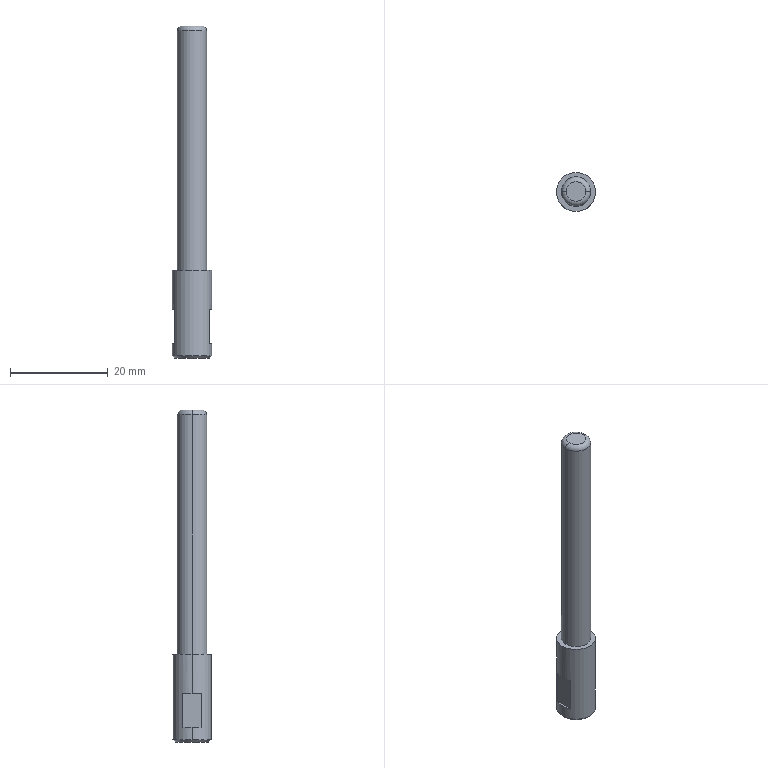Part | SolidWorks | features ICE 2, Chamfer 1, Extrusion 1, Fillet 1, HoleWzd 1 | 1 solid | 21 faces | box 8 x 8 x 68 mm | volume 2175 mm3 | plane 9 | cylinder 6 | cone 4 | torus 2 | commonest cylinder face diameters 3.3 x2 6 x2 8 x2
STEP:
#1=CARTESIAN_POINT('',(1.65,0.,13.5));
#2=VERTEX_POINT('',#1);
#3=CARTESIAN_POINT('',(-1.65,0.,13.5));
#4=VERTEX_POINT('',#3);
#5=CARTESIAN_POINT('',(0.,0.,13.5));
#6=DIRECTION('',(0.,0.,-1.));
#7=DIRECTION('',(-1.,0.,0.));
#8=AXIS2_PLACEMENT_3D('',#5,#6,#7);
#9=CIRCLE('',#8,1.65);
#10=EDGE_CURVE('',#2,#4,#9,.T.);
#11=ORIENTED_EDGE('',*,*,#10,.F.);
#12=CARTESIAN_POINT('',(1.65,0.,0.));
#13=VERTEX_POINT('',#12);
#14=CARTESIAN_POINT('',(1.65,0.,0.));
#15=DIRECTION('',(0.,0.,-1.));
#16=VECTOR('',#15,1000.);
#17=LINE('',#14,#16);
#18=EDGE_CURVE('',#2,#13,#17,.T.);
#19=ORIENTED_EDGE('',*,*,#18,.T.);
#20=CARTESIAN_POINT('',(-1.65,0.,0.));
#21=VERTEX_POINT('',#20);
#22=CARTESIAN_POINT('',(0.,0.,0.));
#23=DIRECTION('',(0.,0.,-1.));
#24=DIRECTION('',(-1.,0.,0.));
#25=AXIS2_PLACEMENT_3D('',#22,#23,#24);
#26=CIRCLE('',#25,1.65);
#27=EDGE_CURVE('',#13,#21,#26,.T.);
#28=ORIENTED_EDGE('',*,*,#27,.T.);
#29=CARTESIAN_POINT('',(-1.65,0.,0.));
#30=DIRECTION('',(0.,0.,-1.));
#31=VECTOR('',#30,1000.);
#32=LINE('',#29,#31);
#33=EDGE_CURVE('',#4,#21,#32,.T.);
#34=ORIENTED_EDGE('',*,*,#33,.F.);
#35=EDGE_LOOP('',(#11,#19,#28,#34));
#36=FACE_OUTER_BOUND('',#35,.T.);
#37=CARTESIAN_POINT('',(0.,0.,0.));
#38=DIRECTION('',(0.,0.,-1.));
#39=DIRECTION('',(-1.,0.,0.));
#40=AXIS2_PLACEMENT_3D('',#37,#38,#39);
#41=CYLINDRICAL_SURFACE('',#40,1.65);
#42=ADVANCED_FACE('',(#36),#41,.F.);
#43=CARTESIAN_POINT('',(0.,0.,14.491));
#44=VERTEX_POINT('',#43);
#45=CARTESIAN_POINT('',(-1.65,0.,13.5));
#46=DIRECTION('',(-0.8572,0.,-0.515));
#47=VECTOR('',#46,1000.);
#48=LINE('',#45,#47);
#49=EDGE_CURVE('',#44,#4,#48,.T.);
#50=ORIENTED_EDGE('',*,*,#49,.F.);
#51=CARTESIAN_POINT('',(1.65,0.,13.5));
#52=DIRECTION('',(0.8572,0.,-0.515));
#53=VECTOR('',#52,1000.);
#54=LINE('',#51,#53);
#55=EDGE_CURVE('',#44,#2,#54,.T.);
#56=ORIENTED_EDGE('',*,*,#55,.T.);
#57=ORIENTED_EDGE('',*,*,#10,.T.);
#58=EDGE_LOOP('',(#50,#56,#57));
#59=FACE_OUTER_BOUND('',#58,.T.);
#60=CARTESIAN_POINT('',(0.,0.,13.5));
#61=DIRECTION('',(0.,0.,-1.));
#62=DIRECTION('',(-1.,0.,0.));
#63=AXIS2_PLACEMENT_3D('',#60,#61,#62);
#64=CONICAL_SURFACE('',#63,1.65,1.03);
#65=ADVANCED_FACE('',(#59),#64,.F.);
#66=CARTESIAN_POINT('',(-3.5,0.,0.));
#67=VERTEX_POINT('',#66);
#68=CARTESIAN_POINT('',(3.5,0.,0.));
#69=VERTEX_POINT('',#68);
#70=CARTESIAN_POINT('',(0.,0.,0.));
#71=DIRECTION('',(0.,0.,-1.));
#72=DIRECTION('',(1.,0.,0.));
#73=AXIS2_PLACEMENT_3D('',#70,#71,#72);
#74=CIRCLE('',#73,3.5);
#75=EDGE_CURVE('',#67,#69,#74,.T.);
#76=ORIENTED_EDGE('',*,*,#75,.F.);
#77=CARTESIAN_POINT('',(-4.,0.,0.5));
#78=VERTEX_POINT('',#77);
#79=CARTESIAN_POINT('',(-4.,0.,0.5));
#80=DIRECTION('',(-0.7071,0.,0.7071));
#81=VECTOR('',#80,1000.);
#82=LINE('',#79,#81);
#83=EDGE_CURVE('',#67,#78,#82,.T.);
#84=ORIENTED_EDGE('',*,*,#83,.T.);
#85=CARTESIAN_POINT('',(4.,0.,0.5));
#86=VERTEX_POINT('',#85);
#87=CARTESIAN_POINT('',(0.,0.,0.5));
#88=DIRECTION('',(0.,0.,1.));
#89=DIRECTION('',(1.,0.,0.));
#90=AXIS2_PLACEMENT_3D('',#87,#88,#89);
#91=CIRCLE('',#90,4.);
#92=EDGE_CURVE('',#86,#78,#91,.T.);
#93=ORIENTED_EDGE('',*,*,#92,.F.);
#94=CARTESIAN_POINT('',(4.,0.,0.5));
#95=DIRECTION('',(0.7071,0.,0.7071));
#96=VECTOR('',#95,1000.);
#97=LINE('',#94,#96);
#98=EDGE_CURVE('',#69,#86,#97,.T.);
#99=ORIENTED_EDGE('',*,*,#98,.F.);
#100=EDGE_LOOP('',(#76,#84,#93,#99));
#101=FACE_OUTER_BOUND('',#100,.T.);
#102=CARTESIAN_POINT('',(0.,0.,0.5));
#103=DIRECTION('',(0.,0.,1.));
#104=DIRECTION('',(1.,0.,0.));
#105=AXIS2_PLACEMENT_3D('',#102,#103,#104);
#106=CONICAL_SURFACE('',#105,4.,0.7854);
#107=ADVANCED_FACE('',(#101),#106,.T.);
#108=CARTESIAN_POINT('',(-3.,0.,67.));
#109=VERTEX_POINT('',#108);
#110=CARTESIAN_POINT('',(3.,0.,67.));
#111=VERTEX_POINT('',#110);
#112=CARTESIAN_POINT('',(0.,0.,67.));
#113=DIRECTION('',(0.,0.,-1.));
#114=DIRECTION('',(1.,0.,0.));
#115=AXIS2_PLACEMENT_3D('',#112,#113,#114);
#116=CIRCLE('',#115,3.);
#117=EDGE_CURVE('',#109,#111,#116,.T.);
#118=ORIENTED_EDGE('',*,*,#117,.F.);
#119=CARTESIAN_POINT('',(-2.,0.,68.));
#120=VERTEX_POINT('',#119);
#121=CARTESIAN_POINT('',(-2.,0.,67.));
#122=DIRECTION('',(0.,1.,0.));
#123=DIRECTION('',(-1.,0.,0.));
#124=AXIS2_PLACEMENT_3D('',#121,#122,#123);
#125=CIRCLE('',#124,1.);
#126=EDGE_CURVE('',#109,#120,#125,.T.);
#127=ORIENTED_EDGE('',*,*,#126,.T.);
#128=CARTESIAN_POINT('',(2.,0.,68.));
#129=VERTEX_POINT('',#128);
#130=CARTESIAN_POINT('',(0.,0.,68.));
#131=DIRECTION('',(0.,0.,1.));
#132=DIRECTION('',(1.,0.,0.));
#133=AXIS2_PLACEMENT_3D('',#130,#131,#132);
#134=CIRCLE('',#133,2.);
#135=EDGE_CURVE('',#129,#120,#134,.T.);
#136=ORIENTED_EDGE('',*,*,#135,.F.);
#137=CARTESIAN_POINT('',(2.,0.,67.));
#138=DIRECTION('',(0.,-1.,0.));
#139=DIRECTION('',(0.,0.,-1.));
#140=AXIS2_PLACEMENT_3D('',#137,#138,#139);
#141=CIRCLE('',#140,1.);
#142=EDGE_CURVE('',#111,#129,#141,.T.);
#143=ORIENTED_EDGE('',*,*,#142,.F.);
#144=EDGE_LOOP('',(#118,#127,#136,#143));
#145=FACE_OUTER_BOUND('',#144,.T.);
#146=CARTESIAN_POINT('',(0.,0.,67.));
#147=DIRECTION('',(0.,0.,1.));
#148=DIRECTION('',(1.,0.,0.));
#149=AXIS2_PLACEMENT_3D('',#146,#147,#148);
#150=TOROIDAL_SURFACE('',#149,2.,1.);
#151=ADVANCED_FACE('',(#145),#150,.T.);
#152=ORIENTED_EDGE('',*,*,#117,.T.);
#153=CARTESIAN_POINT('',(3.,0.,18.));
#154=VERTEX_POINT('',#153);
#155=CARTESIAN_POINT('',(3.,0.,68.));
#156=DIRECTION('',(0.,0.,-1.));
#157=VECTOR('',#156,1000.);
#158=LINE('',#155,#157);
#159=EDGE_CURVE('',#111,#154,#158,.T.);
#160=ORIENTED_EDGE('',*,*,#159,.T.);
#161=CARTESIAN_POINT('',(-3.,0.,18.));
#162=VERTEX_POINT('',#161);
#163=CARTESIAN_POINT('',(0.,0.,18.));
#164=DIRECTION('',(0.,0.,1.));
#165=DIRECTION('',(1.,0.,0.));
#166=AXIS2_PLACEMENT_3D('',#163,#164,#165);
#167=CIRCLE('',#166,3.);
#168=EDGE_CURVE('',#154,#162,#167,.T.);
#169=ORIENTED_EDGE('',*,*,#168,.T.);
#170=CARTESIAN_POINT('',(-3.,0.,68.));
#171=DIRECTION('',(0.,0.,-1.));
#172=VECTOR('',#171,1000.);
#173=LINE('',#170,#172);
#174=EDGE_CURVE('',#109,#162,#173,.T.);
#175=ORIENTED_EDGE('',*,*,#174,.F.);
#176=EDGE_LOOP('',(#152,#160,#169,#175));
#177=FACE_OUTER_BOUND('',#176,.T.);
#178=CARTESIAN_POINT('',(0.,0.,68.));
#179=DIRECTION('',(0.,0.,-1.));
#180=DIRECTION('',(-1.,0.,0.));
#181=AXIS2_PLACEMENT_3D('',#178,#179,#180);
#182=CYLINDRICAL_SURFACE('',#181,3.);
#183=ADVANCED_FACE('',(#177),#182,.T.);
#184=CARTESIAN_POINT('',(4.,0.,18.));
#185=VERTEX_POINT('',#184);
#186=CARTESIAN_POINT('',(-4.,0.,18.));
#187=VERTEX_POINT('',#186);
#188=CARTESIAN_POINT('',(0.,0.,18.));
#189=DIRECTION('',(0.,0.,1.));
#190=DIRECTION('',(1.,0.,0.));
#191=AXIS2_PLACEMENT_3D('',#188,#189,#190);
#192=CIRCLE('',#191,4.);
#193=EDGE_CURVE('',#185,#187,#192,.T.);
#194=ORIENTED_EDGE('',*,*,#193,.F.);
#195=CARTESIAN_POINT('',(4.,0.,10.));
#196=VERTEX_POINT('',#195);
#197=CARTESIAN_POINT('',(4.,0.,18.));
#198=DIRECTION('',(0.,0.,-1.));
#199=VECTOR('',#198,1000.);
#200=LINE('',#197,#199);
#201=EDGE_CURVE('',#185,#196,#200,.T.);
#202=ORIENTED_EDGE('',*,*,#201,.T.);
#203=CARTESIAN_POINT('',(3.5,1.936,10.));
#204=VERTEX_POINT('',#203);
#205=CARTESIAN_POINT('',(0.,0.,10.));
#206=DIRECTION('',(0.,0.,-1.));
#207=DIRECTION('',(-1.,0.,0.));
#208=AXIS2_PLACEMENT_3D('',#205,#206,#207);
#209=CIRCLE('',#208,4.);
#210=EDGE_CURVE('',#204,#196,#209,.T.);
#211=ORIENTED_EDGE('',*,*,#210,.F.);
#212=CARTESIAN_POINT('',(3.5,1.936,3.));
#213=VERTEX_POINT('',#212);
#214=CARTESIAN_POINT('',(3.5,1.936,18.));
#215=DIRECTION('',(0.,0.,-1.));
#216=VECTOR('',#215,1000.);
#217=LINE('',#214,#216);
#218=EDGE_CURVE('',#204,#213,#217,.T.);
#219=ORIENTED_EDGE('',*,*,#218,.T.);
#220=CARTESIAN_POINT('',(4.,0.,3.));
#221=VERTEX_POINT('',#220);
#222=CARTESIAN_POINT('',(0.,0.,3.));
#223=DIRECTION('',(0.,0.,-1.));
#224=DIRECTION('',(-1.,0.,0.));
#225=AXIS2_PLACEMENT_3D('',#222,#223,#224);
#226=CIRCLE('',#225,4.);
#227=EDGE_CURVE('',#213,#221,#226,.T.);
#228=ORIENTED_EDGE('',*,*,#227,.T.);
#229=CARTESIAN_POINT('',(4.,0.,18.));
#230=DIRECTION('',(0.,0.,-1.));
#231=VECTOR('',#230,1000.);
#232=LINE('',#229,#231);
#233=EDGE_CURVE('',#221,#86,#232,.T.);
#234=ORIENTED_EDGE('',*,*,#233,.T.);
#235=ORIENTED_EDGE('',*,*,#92,.T.);
#236=CARTESIAN_POINT('',(-4.,0.,3.));
#237=VERTEX_POINT('',#236);
#238=CARTESIAN_POINT('',(-4.,0.,18.));
#239=DIRECTION('',(0.,0.,-1.));
#240=VECTOR('',#239,1000.);
#241=LINE('',#238,#240);
#242=EDGE_CURVE('',#237,#78,#241,.T.);
#243=ORIENTED_EDGE('',*,*,#242,.F.);
#244=CARTESIAN_POINT('',(-3.5,1.936,3.));
#245=VERTEX_POINT('',#244);
#246=CARTESIAN_POINT('',(0.,0.,3.));
#247=DIRECTION('',(0.,0.,-1.));
#248=DIRECTION('',(-1.,0.,0.));
#249=AXIS2_PLACEMENT_3D('',#246,#247,#248);
#250=CIRCLE('',#249,4.);
#251=EDGE_CURVE('',#237,#245,#250,.T.);
#252=ORIENTED_EDGE('',*,*,#251,.T.);
#253=CARTESIAN_POINT('',(-3.5,1.936,10.));
#254=VERTEX_POINT('',#253);
#255=CARTESIAN_POINT('',(-3.5,1.936,18.));
#256=DIRECTION('',(0.,0.,1.));
#257=VECTOR('',#256,1000.);
#258=LINE('',#255,#257);
#259=EDGE_CURVE('',#245,#254,#258,.T.);
#260=ORIENTED_EDGE('',*,*,#259,.T.);
#261=CARTESIAN_POINT('',(-4.,0.,10.));
#262=VERTEX_POINT('',#261);
#263=CARTESIAN_POINT('',(0.,0.,10.));
#264=DIRECTION('',(0.,0.,-1.));
#265=DIRECTION('',(-1.,0.,0.));
#266=AXIS2_PLACEMENT_3D('',#263,#264,#265);
#267=CIRCLE('',#266,4.);
#268=EDGE_CURVE('',#262,#254,#267,.T.);
#269=ORIENTED_EDGE('',*,*,#268,.F.);
#270=CARTESIAN_POINT('',(-4.,0.,18.));
#271=DIRECTION('',(0.,0.,-1.));
#272=VECTOR('',#271,1000.);
#273=LINE('',#270,#272);
#274=EDGE_CURVE('',#187,#262,#273,.T.);
#275=ORIENTED_EDGE('',*,*,#274,.F.);
#276=EDGE_LOOP('',(#194,#202,#211,#219,#228,#234,#235,#243,#252,#260,#269,#275));
#277=FACE_OUTER_BOUND('',#276,.T.);
#278=CARTESIAN_POINT('',(0.,0.,18.));
#279=DIRECTION('',(0.,0.,-1.));
#280=DIRECTION('',(-1.,0.,0.));
#281=AXIS2_PLACEMENT_3D('',#278,#279,#280);
#282=CYLINDRICAL_SURFACE('',#281,4.);
#283=ADVANCED_FACE('',(#277),#282,.T.);
#284=ORIENTED_EDGE('',*,*,#201,.F.);
#285=CARTESIAN_POINT('',(0.,0.,18.));
#286=DIRECTION('',(0.,0.,1.));
#287=DIRECTION('',(1.,0.,0.));
#288=AXIS2_PLACEMENT_3D('',#285,#286,#287);
#289=CIRCLE('',#288,4.);
#290=EDGE_CURVE('',#187,#185,#289,.T.);
#291=ORIENTED_EDGE('',*,*,#290,.F.);
#292=ORIENTED_EDGE('',*,*,#274,.T.);
#293=CARTESIAN_POINT('',(-3.5,-1.936,10.));
#294=VERTEX_POINT('',#293);
#295=CARTESIAN_POINT('',(0.,0.,10.));
#296=DIRECTION('',(0.,0.,-1.));
#297=DIRECTION('',(-1.,0.,0.));
#298=AXIS2_PLACEMENT_3D('',#295,#296,#297);
#299=CIRCLE('',#298,4.);
#300=EDGE_CURVE('',#294,#262,#299,.T.);
#301=ORIENTED_EDGE('',*,*,#300,.F.);
#302=CARTESIAN_POINT('',(-3.5,-1.936,3.));
#303=VERTEX_POINT('',#302);
#304=CARTESIAN_POINT('',(-3.5,-1.936,18.));
#305=DIRECTION('',(0.,0.,-1.));
#306=VECTOR('',#305,1000.);
#307=LINE('',#304,#306);
#308=EDGE_CURVE('',#294,#303,#307,.T.);
#309=ORIENTED_EDGE('',*,*,#308,.T.);
#310=CARTESIAN_POINT('',(0.,0.,3.));
#311=DIRECTION('',(0.,0.,-1.));
#312=DIRECTION('',(-1.,0.,0.));
#313=AXIS2_PLACEMENT_3D('',#310,#311,#312);
#314=CIRCLE('',#313,4.);
#315=EDGE_CURVE('',#303,#237,#314,.T.);
#316=ORIENTED_EDGE('',*,*,#315,.T.);
#317=ORIENTED_EDGE('',*,*,#242,.T.);
#318=CARTESIAN_POINT('',(0.,0.,0.5));
#319=DIRECTION('',(0.,0.,1.));
#320=DIRECTION('',(1.,0.,0.));
#321=AXIS2_PLACEMENT_3D('',#318,#319,#320);
#322=CIRCLE('',#321,4.);
#323=EDGE_CURVE('',#78,#86,#322,.T.);
#324=ORIENTED_EDGE('',*,*,#323,.T.);
#325=ORIENTED_EDGE('',*,*,#233,.F.);
#326=CARTESIAN_POINT('',(3.5,-1.936,3.));
#327=VERTEX_POINT('',#326);
#328=CARTESIAN_POINT('',(0.,0.,3.));
#329=DIRECTION('',(0.,0.,-1.));
#330=DIRECTION('',(-1.,0.,0.));
#331=AXIS2_PLACEMENT_3D('',#328,#329,#330);
#332=CIRCLE('',#331,4.);
#333=EDGE_CURVE('',#221,#327,#332,.T.);
#334=ORIENTED_EDGE('',*,*,#333,.T.);
#335=CARTESIAN_POINT('',(3.5,-1.936,10.));
#336=VERTEX_POINT('',#335);
#337=CARTESIAN_POINT('',(3.5,-1.936,18.));
#338=DIRECTION('',(0.,0.,1.));
#339=VECTOR('',#338,1000.);
#340=LINE('',#337,#339);
#341=EDGE_CURVE('',#327,#336,#340,.T.);
#342=ORIENTED_EDGE('',*,*,#341,.T.);
#343=CARTESIAN_POINT('',(0.,0.,10.));
#344=DIRECTION('',(0.,0.,-1.));
#345=DIRECTION('',(-1.,0.,0.));
#346=AXIS2_PLACEMENT_3D('',#343,#344,#345);
#347=CIRCLE('',#346,4.);
#348=EDGE_CURVE('',#196,#336,#347,.T.);
#349=ORIENTED_EDGE('',*,*,#348,.F.);
#350=EDGE_LOOP('',(#284,#291,#292,#301,#309,#316,#317,#324,#325,#334,#342,#349));
#351=FACE_OUTER_BOUND('',#350,.T.);
#352=CARTESIAN_POINT('',(0.,0.,18.));
#353=DIRECTION('',(0.,0.,-1.));
#354=DIRECTION('',(-1.,0.,0.));
#355=AXIS2_PLACEMENT_3D('',#352,#353,#354);
#356=CYLINDRICAL_SURFACE('',#355,4.);
#357=ADVANCED_FACE('',(#351),#356,.T.);
#358=CARTESIAN_POINT('',(0.,0.,18.));
#359=DIRECTION('',(0.,0.,1.));
#360=DIRECTION('',(1.,0.,0.));
#361=AXIS2_PLACEMENT_3D('',#358,#359,#360);
#362=CIRCLE('',#361,3.);
#363=EDGE_CURVE('',#162,#154,#362,.T.);
#364=ORIENTED_EDGE('',*,*,#363,.F.);
#365=ORIENTED_EDGE('',*,*,#168,.F.);
#366=EDGE_LOOP('',(#364,#365));
#367=FACE_BOUND('',#366,.T.);
#368=ORIENTED_EDGE('',*,*,#290,.T.);
#369=ORIENTED_EDGE('',*,*,#193,.T.);
#370=EDGE_LOOP('',(#368,#369));
#371=FACE_OUTER_BOUND('',#370,.T.);
#372=CARTESIAN_POINT('',(0.,0.,18.));
#373=DIRECTION('',(0.,0.,1.));
#374=DIRECTION('',(1.,0.,0.));
#375=AXIS2_PLACEMENT_3D('',#372,#373,#374);
#376=PLANE('',#375);
#377=ADVANCED_FACE('',(#367,#371),#376,.T.);
#378=CARTESIAN_POINT('',(0.,0.,0.));
#379=DIRECTION('',(0.,0.,-1.));
#380=DIRECTION('',(-1.,0.,0.));
#381=AXIS2_PLACEMENT_3D('',#378,#379,#380);
#382=CIRCLE('',#381,1.65);
#383=EDGE_CURVE('',#21,#13,#382,.T.);
#384=ORIENTED_EDGE('',*,*,#383,.F.);
#385=ORIENTED_EDGE('',*,*,#27,.F.);
#386=EDGE_LOOP('',(#384,#385));
#387=FACE_BOUND('',#386,.T.);
#388=CARTESIAN_POINT('',(0.,0.,0.));
#389=DIRECTION('',(0.,0.,-1.));
#390=DIRECTION('',(1.,0.,0.));
#391=AXIS2_PLACEMENT_3D('',#388,#389,#390);
#392=CIRCLE('',#391,3.5);
#393=EDGE_CURVE('',#69,#67,#392,.T.);
#394=ORIENTED_EDGE('',*,*,#393,.T.);
#395=ORIENTED_EDGE('',*,*,#75,.T.);
#396=EDGE_LOOP('',(#394,#395));
#397=FACE_OUTER_BOUND('',#396,.T.);
#398=CARTESIAN_POINT('',(0.,0.,0.));
#399=DIRECTION('',(0.,0.,1.));
#400=DIRECTION('',(1.,0.,0.));
#401=AXIS2_PLACEMENT_3D('',#398,#399,#400);
#402=PLANE('',#401);
#403=ADVANCED_FACE('',(#387,#397),#402,.F.);
#404=ORIENTED_EDGE('',*,*,#159,.F.);
#405=CARTESIAN_POINT('',(0.,0.,67.));
#406=DIRECTION('',(0.,0.,-1.));
#407=DIRECTION('',(1.,0.,0.));
#408=AXIS2_PLACEMENT_3D('',#405,#406,#407);
#409=CIRCLE('',#408,3.);
#410=EDGE_CURVE('',#111,#109,#409,.T.);
#411=ORIENTED_EDGE('',*,*,#410,.T.);
#412=ORIENTED_EDGE('',*,*,#174,.T.);
#413=ORIENTED_EDGE('',*,*,#363,.T.);
#414=EDGE_LOOP('',(#404,#411,#412,#413));
#415=FACE_OUTER_BOUND('',#414,.T.);
#416=CARTESIAN_POINT('',(0.,0.,68.));
#417=DIRECTION('',(0.,0.,-1.));
#418=DIRECTION('',(-1.,0.,0.));
#419=AXIS2_PLACEMENT_3D('',#416,#417,#418);
#420=CYLINDRICAL_SURFACE('',#419,3.);
#421=ADVANCED_FACE('',(#415),#420,.T.);
#422=ORIENTED_EDGE('',*,*,#135,.T.);
#423=CARTESIAN_POINT('',(0.,0.,68.));
#424=DIRECTION('',(0.,0.,1.));
#425=DIRECTION('',(1.,0.,0.));
#426=AXIS2_PLACEMENT_3D('',#423,#424,#425);
#427=CIRCLE('',#426,2.);
#428=EDGE_CURVE('',#120,#129,#427,.T.);
#429=ORIENTED_EDGE('',*,*,#428,.T.);
#430=EDGE_LOOP('',(#422,#429));
#431=FACE_OUTER_BOUND('',#430,.T.);
#432=CARTESIAN_POINT('',(0.,0.,68.));
#433=DIRECTION('',(0.,0.,1.));
#434=DIRECTION('',(1.,0.,0.));
#435=AXIS2_PLACEMENT_3D('',#432,#433,#434);
#436=PLANE('',#435);
#437=ADVANCED_FACE('',(#431),#436,.T.);
#438=ORIENTED_EDGE('',*,*,#126,.F.);
#439=ORIENTED_EDGE('',*,*,#410,.F.);
#440=ORIENTED_EDGE('',*,*,#142,.T.);
#441=ORIENTED_EDGE('',*,*,#428,.F.);
#442=EDGE_LOOP('',(#438,#439,#440,#441));
#443=FACE_OUTER_BOUND('',#442,.T.);
#444=CARTESIAN_POINT('',(0.,0.,67.));
#445=DIRECTION('',(0.,0.,1.));
#446=DIRECTION('',(1.,0.,0.));
#447=AXIS2_PLACEMENT_3D('',#444,#445,#446);
#448=TOROIDAL_SURFACE('',#447,2.,1.);
#449=ADVANCED_FACE('',(#443),#448,.T.);
#450=ORIENTED_EDGE('',*,*,#83,.F.);
#451=ORIENTED_EDGE('',*,*,#393,.F.);
#452=ORIENTED_EDGE('',*,*,#98,.T.);
#453=ORIENTED_EDGE('',*,*,#323,.F.);
#454=EDGE_LOOP('',(#450,#451,#452,#453));
#455=FACE_OUTER_BOUND('',#454,.T.);
#456=CARTESIAN_POINT('',(0.,0.,0.5));
#457=DIRECTION('',(0.,0.,1.));
#458=DIRECTION('',(1.,0.,0.));
#459=AXIS2_PLACEMENT_3D('',#456,#457,#458);
#460=CONICAL_SURFACE('',#459,4.,0.7854);
#461=ADVANCED_FACE('',(#455),#460,.T.);
#462=ORIENTED_EDGE('',*,*,#55,.F.);
#463=ORIENTED_EDGE('',*,*,#49,.T.);
#464=CARTESIAN_POINT('',(0.,0.,13.5));
#465=DIRECTION('',(0.,0.,-1.));
#466=DIRECTION('',(-1.,0.,0.));
#467=AXIS2_PLACEMENT_3D('',#464,#465,#466);
#468=CIRCLE('',#467,1.65);
#469=EDGE_CURVE('',#4,#2,#468,.T.);
#470=ORIENTED_EDGE('',*,*,#469,.T.);
#471=EDGE_LOOP('',(#462,#463,#470));
#472=FACE_OUTER_BOUND('',#471,.T.);
#473=CARTESIAN_POINT('',(0.,0.,13.5));
#474=DIRECTION('',(0.,0.,-1.));
#475=DIRECTION('',(-1.,0.,0.));
#476=AXIS2_PLACEMENT_3D('',#473,#474,#475);
#477=CONICAL_SURFACE('',#476,1.65,1.03);
#478=ADVANCED_FACE('',(#472),#477,.F.);
#479=ORIENTED_EDGE('',*,*,#18,.F.);
#480=ORIENTED_EDGE('',*,*,#469,.F.);
#481=ORIENTED_EDGE('',*,*,#33,.T.);
#482=ORIENTED_EDGE('',*,*,#383,.T.);
#483=EDGE_LOOP('',(#479,#480,#481,#482));
#484=FACE_OUTER_BOUND('',#483,.T.);
#485=CARTESIAN_POINT('',(0.,0.,0.));
#486=DIRECTION('',(0.,0.,-1.));
#487=DIRECTION('',(-1.,0.,0.));
#488=AXIS2_PLACEMENT_3D('',#485,#486,#487);
#489=CYLINDRICAL_SURFACE('',#488,1.65);
#490=ADVANCED_FACE('',(#484),#489,.F.);
#491=CARTESIAN_POINT('',(3.5,4.545,10.));
#492=DIRECTION('',(0.,1.,0.));
#493=VECTOR('',#492,1000.);
#494=LINE('',#491,#493);
#495=EDGE_CURVE('',#336,#204,#494,.T.);
#496=ORIENTED_EDGE('',*,*,#495,.F.);
#497=ORIENTED_EDGE('',*,*,#341,.F.);
#498=CARTESIAN_POINT('',(3.5,4.545,3.));
#499=DIRECTION('',(0.,1.,0.));
#500=VECTOR('',#499,1000.);
#501=LINE('',#498,#500);
#502=EDGE_CURVE('',#327,#213,#501,.T.);
#503=ORIENTED_EDGE('',*,*,#502,.T.);
#504=ORIENTED_EDGE('',*,*,#218,.F.);
#505=EDGE_LOOP('',(#496,#497,#503,#504));
#506=FACE_OUTER_BOUND('',#505,.T.);
#507=CARTESIAN_POINT('',(3.5,4.545,10.));
#508=DIRECTION('',(-1.,0.,0.));
#509=DIRECTION('',(0.,-1.,0.));
#510=AXIS2_PLACEMENT_3D('',#507,#508,#509);
#511=PLANE('',#510);
#512=ADVANCED_FACE('',(#506),#511,.F.);
#513=ORIENTED_EDGE('',*,*,#210,.T.);
#514=ORIENTED_EDGE('',*,*,#348,.T.);
#515=ORIENTED_EDGE('',*,*,#495,.T.);
#516=EDGE_LOOP('',(#513,#514,#515));
#517=FACE_OUTER_BOUND('',#516,.T.);
#518=CARTESIAN_POINT('',(0.,0.,10.));
#519=DIRECTION('',(0.,0.,-1.));
#520=DIRECTION('',(-1.,0.,0.));
#521=AXIS2_PLACEMENT_3D('',#518,#519,#520);
#522=PLANE('',#521);
#523=ADVANCED_FACE('',(#517),#522,.T.);
#524=ORIENTED_EDGE('',*,*,#502,.F.);
#525=ORIENTED_EDGE('',*,*,#333,.F.);
#526=ORIENTED_EDGE('',*,*,#227,.F.);
#527=EDGE_LOOP('',(#524,#525,#526));
#528=FACE_OUTER_BOUND('',#527,.T.);
#529=CARTESIAN_POINT('',(0.,0.,3.));
#530=DIRECTION('',(0.,0.,-1.));
#531=DIRECTION('',(-1.,0.,0.));
#532=AXIS2_PLACEMENT_3D('',#529,#530,#531);
#533=PLANE('',#532);
#534=ADVANCED_FACE('',(#528),#533,.F.);
#535=CARTESIAN_POINT('',(-3.5,4.545,10.));
#536=DIRECTION('',(0.,-1.,0.));
#537=VECTOR('',#536,1000.);
#538=LINE('',#535,#537);
#539=EDGE_CURVE('',#254,#294,#538,.T.);
#540=ORIENTED_EDGE('',*,*,#539,.F.);
#541=ORIENTED_EDGE('',*,*,#259,.F.);
#542=CARTESIAN_POINT('',(-3.5,4.545,3.));
#543=DIRECTION('',(0.,-1.,0.));
#544=VECTOR('',#543,1000.);
#545=LINE('',#542,#544);
#546=EDGE_CURVE('',#245,#303,#545,.T.);
#547=ORIENTED_EDGE('',*,*,#546,.T.);
#548=ORIENTED_EDGE('',*,*,#308,.F.);
#549=EDGE_LOOP('',(#540,#541,#547,#548));
#550=FACE_OUTER_BOUND('',#549,.T.);
#551=CARTESIAN_POINT('',(-3.5,4.545,10.));
#552=DIRECTION('',(1.,0.,0.));
#553=DIRECTION('',(0.,1.,0.));
#554=AXIS2_PLACEMENT_3D('',#551,#552,#553);
#555=PLANE('',#554);
#556=ADVANCED_FACE('',(#550),#555,.F.);
#557=ORIENTED_EDGE('',*,*,#300,.T.);
#558=ORIENTED_EDGE('',*,*,#268,.T.);
#559=ORIENTED_EDGE('',*,*,#539,.T.);
#560=EDGE_LOOP('',(#557,#558,#559));
#561=FACE_OUTER_BOUND('',#560,.T.);
#562=CARTESIAN_POINT('',(0.,0.,10.));
#563=DIRECTION('',(0.,0.,-1.));
#564=DIRECTION('',(-1.,0.,0.));
#565=AXIS2_PLACEMENT_3D('',#562,#563,#564);
#566=PLANE('',#565);
#567=ADVANCED_FACE('',(#561),#566,.T.);
#568=ORIENTED_EDGE('',*,*,#546,.F.);
#569=ORIENTED_EDGE('',*,*,#251,.F.);
#570=ORIENTED_EDGE('',*,*,#315,.F.);
#571=EDGE_LOOP('',(#568,#569,#570));
#572=FACE_OUTER_BOUND('',#571,.T.);
#573=CARTESIAN_POINT('',(0.,0.,3.));
#574=DIRECTION('',(0.,0.,-1.));
#575=DIRECTION('',(-1.,0.,0.));
#576=AXIS2_PLACEMENT_3D('',#573,#574,#575);
#577=PLANE('',#576);
#578=ADVANCED_FACE('',(#572),#577,.F.);
#579=CLOSED_SHELL('',(#42,#65,#107,#151,#183,#283,#357,#377,#403,#421,#437,#449,#461,#478,#490,#512,#523,#534,#556,#567,#578));
#580=MANIFOLD_SOLID_BREP('',#579);
#581=CARTESIAN_POINT('',(0.,0.,0.));
#582=DIRECTION('',(0.,0.,1.));
#583=DIRECTION('',(1.,0.,0.));
#584=AXIS2_PLACEMENT_3D('',#581,#582,#583);
#585=(LENGTH_UNIT()NAMED_UNIT(*)SI_UNIT(.MILLI.,.METRE.));
#586=UNCERTAINTY_MEASURE_WITH_UNIT(LENGTH_MEASURE(0.00001),#585,'','');
#587=(NAMED_UNIT(*)PLANE_ANGLE_UNIT()SI_UNIT($,.RADIAN.));
#588=(NAMED_UNIT(*)SI_UNIT($,.STERADIAN.)SOLID_ANGLE_UNIT());
#589=(GEOMETRIC_REPRESENTATION_CONTEXT(3)GLOBAL_UNCERTAINTY_ASSIGNED_CONTEXT((#586))GLOBAL_UNIT_ASSIGNED_CONTEXT((#585,#587,#588))REPRESENTATION_CONTEXT('',''));
#590=ADVANCED_BREP_SHAPE_REPRESENTATION('',(#580,#584),#589);